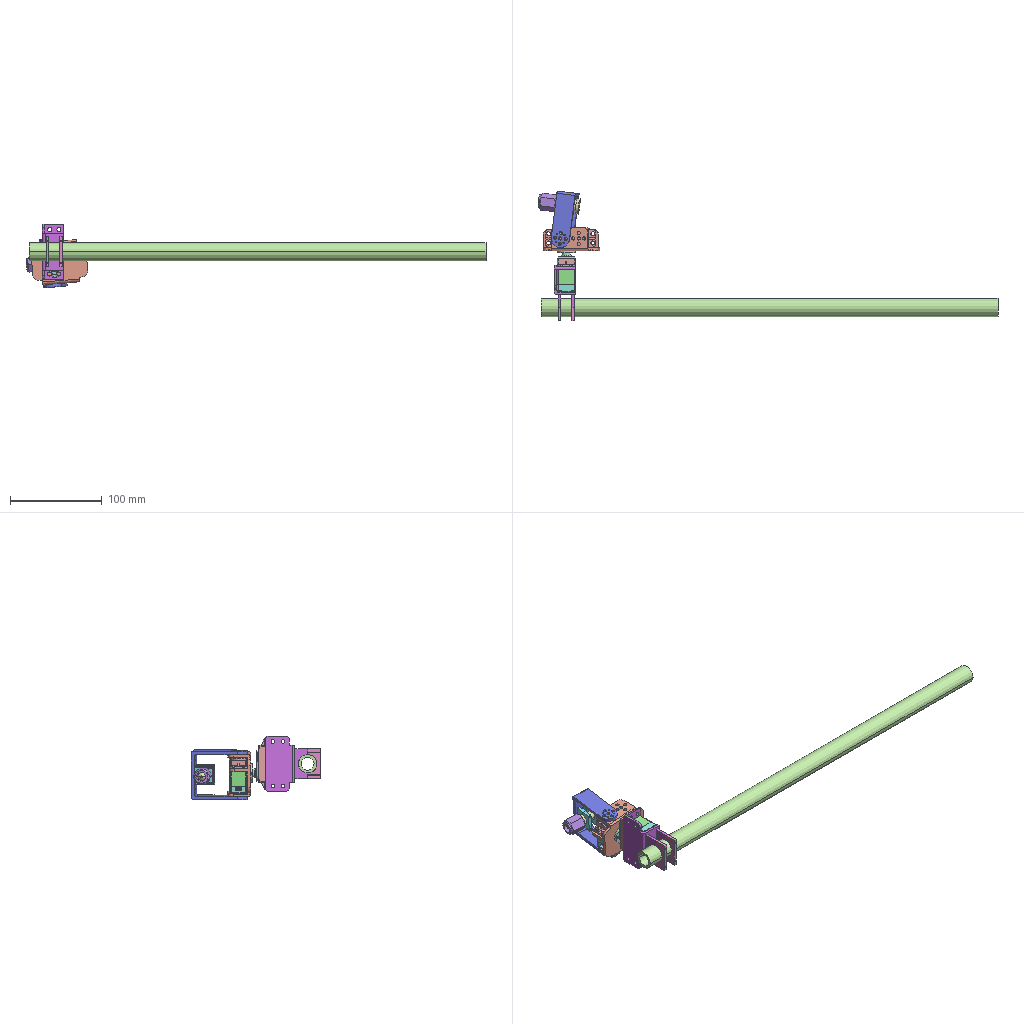Assembly | SolidWorks | 10 different items | 15 placed | box 502 x 141 x 70 mm
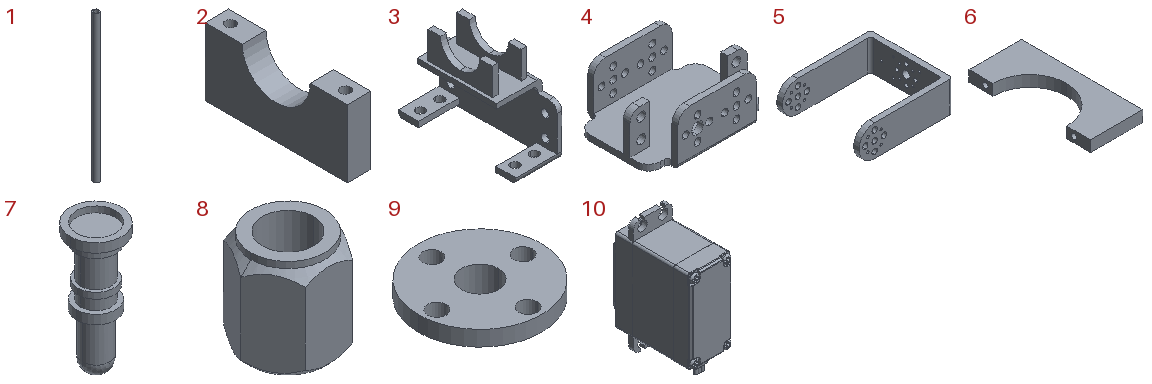Parts list (item | quantity | size | volume | features):
1 | x1 | 20 x 20 x 498 mm | 79790 mm3 | features Cut 1, Extrusion 1
2 | x4 | 3.5 x 21 x 10 mm | 562.212 mm3 | features Cut 2, Extrusion 1
3 | x1 | 23.5 x 60.5 x 46 mm | 9322 mm3 | features ICE 4, Cut 3, Fillet 2, MirrorPattern 2, Extrusion 1
4 | x1 | 60 x 46 x 25 mm | 13187 mm3 | features Fillet 7, Cut 5, ICE 2, Extrusion 1, MirrorPattern 1
5 | x1 | 60.5 x 53 x 20 mm | 10804 mm3 | features Cut 5, Fillet 2, Extrusion 1
6 | x2 | 14.182 x 33 x 3 mm | 882.699 mm3 | features Cut 1, Extrusion 1
7 | x1 | 17 x 17 x 42.888 mm | 3533 mm3 | features ICE 7, Cut 1, Dome 1, Extrusion 1
8 | x1 | 18.475 x 16 x 19.2 mm | 2605 mm3 | features RevCut 2, Extrusion 1, ICE 1
9 | x1 | 20 x 20 x 5 mm | 732.384 mm3 | features Cut 1, Extrusion 1, ICE 1
10 | x2 | 20.1 x 43.6 x 55.6 mm | 25971 mm3 | features BaseBody 11, Cut 1
Mates (type | each side: item.copy, entity, surface, feature):
Coincident | 10.1 plane | assembly plane | 3 times
InPlace | 10.1 face plane Input 5 | 3.1 plane
Concentric | 10.1 face cylinder Input 8 | 9.1 face cylinder Boss-Extrude1
Coincident | 10.1 face plane Input 1 | 9.1 face plane Boss-Extrude1
InPlace | 9.1 face plane Boss-Extrude2 | 4.1 plane
Coincident | 4.1 face plane Boss-Extrude2 | 10.2 face plane Input 9
Coincident | 4.1 face plane Boss-Extrude2 | 10.2 face plane Input 5
InPlace | 3.1 face plane Boss-Extrude2 | 1.1 plane
InPlace | 3.1 face plane Boss-Extrude2 | 6.1 plane
Coincident | 3.1 face plane Boss-Extrude2 | 6.2 face plane Boss-Extrude1 | 3 times
Concentric | 4.1 edge | 5.1 face cylinder Cut-Extrude2
Coincident | 4.1 face plane Mirror2 | 5.1 face plane Boss-Extrude1
Concentric | 5.1 face cylinder Cut-Extrude4 | 2.1 face cylinder Cut-Extrude1 | 2 times
Coincident | 5.1 face plane Boss-Extrude1 | 2.1 face plane Boss-Extrude1
Coincident | 2.1 face plane Boss-Extrude1 | 2.2 face plane Boss-Extrude1
Coincident | 2.1 edge | 2.2 edge
Concentric | 5.1 edge | 2.3 edge
Concentric | 5.1 face cylinder Cut-Extrude4 | 2.3 face cylinder Cut-Extrude1
Coincident | 5.1 face plane Boss-Extrude1 | 2.3 face plane Boss-Extrude1
Coincident | 2.3 face plane Boss-Extrude1 | 2.4 face plane Boss-Extrude1 | 3 times
InPlace | 2.2 face plane Boss-Extrude1 | 7.1 plane
InPlace | 7.1 face plane Boss-Extrude7 | 8.1 plane